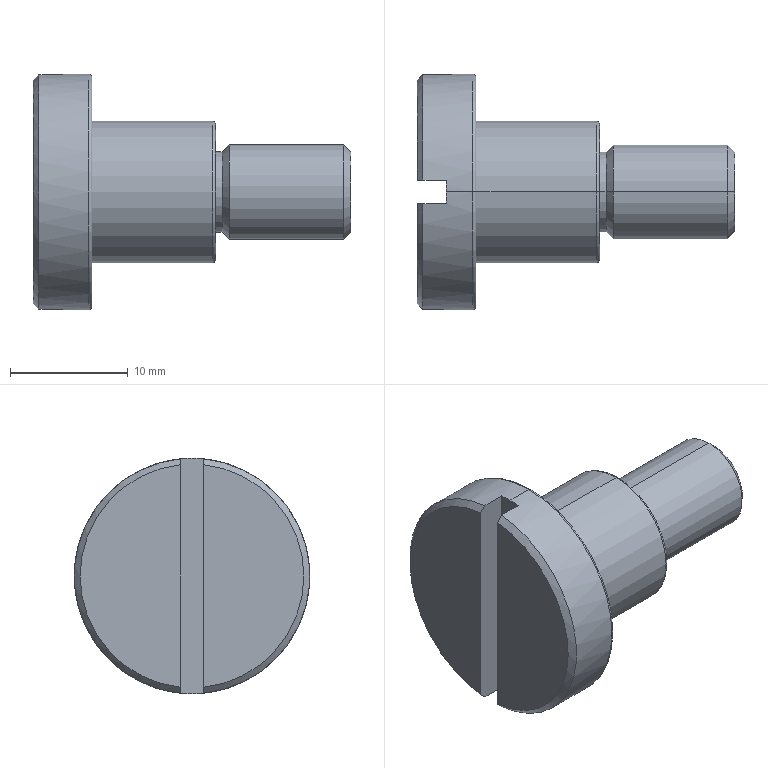Part | SolidWorks | features Chamfer 1, Fillet 1, ICE 1, Revolution 1 | 1 solid | 26 faces | box 27 x 20 x 20 mm | volume 3212 mm3 | cylinder 8 | plane 8 | cone 6 | torus 4 | commonest cylinder face diameters 6.8 x2 8 x2 12 x2 20 x2
STEP:
#1=CARTESIAN_POINT('',(5.,0.,-9.75));
#2=VERTEX_POINT('',#1);
#3=CARTESIAN_POINT('',(5.,0.,9.75));
#4=VERTEX_POINT('',#3);
#5=CARTESIAN_POINT('',(5.,0.,0.));
#6=DIRECTION('',(1.,0.,0.));
#7=DIRECTION('',(0.,0.,1.));
#8=AXIS2_PLACEMENT_3D('',#5,#6,#7);
#9=CIRCLE('',#8,9.75);
#10=EDGE_CURVE('',#2,#4,#9,.T.);
#11=ORIENTED_EDGE('',*,*,#10,.F.);
#12=CARTESIAN_POINT('',(4.75,0.,-10.));
#13=VERTEX_POINT('',#12);
#14=CARTESIAN_POINT('',(4.75,0.,-9.75));
#15=DIRECTION('',(0.,1.,0.));
#16=DIRECTION('',(0.,0.,1.));
#17=AXIS2_PLACEMENT_3D('',#14,#15,#16);
#18=CIRCLE('',#17,0.25);
#19=EDGE_CURVE('',#2,#13,#18,.T.);
#20=ORIENTED_EDGE('',*,*,#19,.T.);
#21=CARTESIAN_POINT('',(4.75,0.,10.));
#22=VERTEX_POINT('',#21);
#23=CARTESIAN_POINT('',(4.75,0.,0.));
#24=DIRECTION('',(-1.,0.,0.));
#25=DIRECTION('',(0.,0.,1.));
#26=AXIS2_PLACEMENT_3D('',#23,#24,#25);
#27=CIRCLE('',#26,10.);
#28=EDGE_CURVE('',#22,#13,#27,.T.);
#29=ORIENTED_EDGE('',*,*,#28,.F.);
#30=CARTESIAN_POINT('',(4.75,0.,9.75));
#31=DIRECTION('',(0.,-1.,0.));
#32=DIRECTION('',(0.,0.,-1.));
#33=AXIS2_PLACEMENT_3D('',#30,#31,#32);
#34=CIRCLE('',#33,0.25);
#35=EDGE_CURVE('',#4,#22,#34,.T.);
#36=ORIENTED_EDGE('',*,*,#35,.F.);
#37=EDGE_LOOP('',(#11,#20,#29,#36));
#38=FACE_OUTER_BOUND('',#37,.T.);
#39=CARTESIAN_POINT('',(4.75,0.,0.));
#40=DIRECTION('',(-1.,0.,0.));
#41=DIRECTION('',(0.,0.,1.));
#42=AXIS2_PLACEMENT_3D('',#39,#40,#41);
#43=TOROIDAL_SURFACE('',#42,9.75,0.25);
#44=ADVANCED_FACE('',(#38),#43,.T.);
#45=CARTESIAN_POINT('',(15.5,0.,-5.75));
#46=VERTEX_POINT('',#45);
#47=CARTESIAN_POINT('',(15.5,0.,5.75));
#48=VERTEX_POINT('',#47);
#49=CARTESIAN_POINT('',(15.5,0.,0.));
#50=DIRECTION('',(1.,0.,0.));
#51=DIRECTION('',(0.,0.,1.));
#52=AXIS2_PLACEMENT_3D('',#49,#50,#51);
#53=CIRCLE('',#52,5.75);
#54=EDGE_CURVE('',#46,#48,#53,.T.);
#55=ORIENTED_EDGE('',*,*,#54,.F.);
#56=CARTESIAN_POINT('',(15.25,0.,-6.));
#57=VERTEX_POINT('',#56);
#58=CARTESIAN_POINT('',(15.25,0.,-5.75));
#59=DIRECTION('',(0.,1.,0.));
#60=DIRECTION('',(0.,0.,1.));
#61=AXIS2_PLACEMENT_3D('',#58,#59,#60);
#62=CIRCLE('',#61,0.25);
#63=EDGE_CURVE('',#46,#57,#62,.T.);
#64=ORIENTED_EDGE('',*,*,#63,.T.);
#65=CARTESIAN_POINT('',(15.25,0.,6.));
#66=VERTEX_POINT('',#65);
#67=CARTESIAN_POINT('',(15.25,0.,0.));
#68=DIRECTION('',(-1.,0.,0.));
#69=DIRECTION('',(0.,0.,1.));
#70=AXIS2_PLACEMENT_3D('',#67,#68,#69);
#71=CIRCLE('',#70,6.);
#72=EDGE_CURVE('',#66,#57,#71,.T.);
#73=ORIENTED_EDGE('',*,*,#72,.F.);
#74=CARTESIAN_POINT('',(15.25,0.,5.75));
#75=DIRECTION('',(0.,-1.,0.));
#76=DIRECTION('',(0.,0.,-1.));
#77=AXIS2_PLACEMENT_3D('',#74,#75,#76);
#78=CIRCLE('',#77,0.25);
#79=EDGE_CURVE('',#48,#66,#78,.T.);
#80=ORIENTED_EDGE('',*,*,#79,.F.);
#81=EDGE_LOOP('',(#55,#64,#73,#80));
#82=FACE_OUTER_BOUND('',#81,.T.);
#83=CARTESIAN_POINT('',(15.25,0.,0.));
#84=DIRECTION('',(-1.,0.,0.));
#85=DIRECTION('',(0.,0.,1.));
#86=AXIS2_PLACEMENT_3D('',#83,#84,#85);
#87=TOROIDAL_SURFACE('',#86,5.75,0.25);
#88=ADVANCED_FACE('',(#82),#87,.T.);
#89=CARTESIAN_POINT('',(27.,0.,3.4));
#90=VERTEX_POINT('',#89);
#91=CARTESIAN_POINT('',(27.,0.,-3.4));
#92=VERTEX_POINT('',#91);
#93=CARTESIAN_POINT('',(27.,0.,0.));
#94=DIRECTION('',(-1.,0.,0.));
#95=DIRECTION('',(0.,0.,1.));
#96=AXIS2_PLACEMENT_3D('',#93,#94,#95);
#97=CIRCLE('',#96,3.4);
#98=EDGE_CURVE('',#90,#92,#97,.T.);
#99=ORIENTED_EDGE('',*,*,#98,.T.);
#100=CARTESIAN_POINT('',(26.4,0.,-4.));
#101=VERTEX_POINT('',#100);
#102=CARTESIAN_POINT('',(27.,0.,-3.4));
#103=DIRECTION('',(-0.7071,0.,-0.7071));
#104=VECTOR('',#103,1000.);
#105=LINE('',#102,#104);
#106=EDGE_CURVE('',#92,#101,#105,.T.);
#107=ORIENTED_EDGE('',*,*,#106,.T.);
#108=CARTESIAN_POINT('',(26.4,0.,4.));
#109=VERTEX_POINT('',#108);
#110=CARTESIAN_POINT('',(26.4,0.,0.));
#111=DIRECTION('',(-1.,0.,0.));
#112=DIRECTION('',(0.,0.,1.));
#113=AXIS2_PLACEMENT_3D('',#110,#111,#112);
#114=CIRCLE('',#113,4.);
#115=EDGE_CURVE('',#109,#101,#114,.T.);
#116=ORIENTED_EDGE('',*,*,#115,.F.);
#117=CARTESIAN_POINT('',(27.,0.,3.4));
#118=DIRECTION('',(-0.7071,0.,0.7071));
#119=VECTOR('',#118,1000.);
#120=LINE('',#117,#119);
#121=EDGE_CURVE('',#90,#109,#120,.T.);
#122=ORIENTED_EDGE('',*,*,#121,.F.);
#123=EDGE_LOOP('',(#99,#107,#116,#122));
#124=FACE_OUTER_BOUND('',#123,.T.);
#125=CARTESIAN_POINT('',(27.,0.,0.));
#126=DIRECTION('',(-1.,0.,0.));
#127=DIRECTION('',(0.,0.,1.));
#128=AXIS2_PLACEMENT_3D('',#125,#126,#127);
#129=CONICAL_SURFACE('',#128,3.4,0.7854);
#130=ADVANCED_FACE('',(#124),#129,.T.);
#131=ORIENTED_EDGE('',*,*,#115,.T.);
#132=CARTESIAN_POINT('',(16.65,0.,-4.));
#133=VERTEX_POINT('',#132);
#134=CARTESIAN_POINT('',(0.,0.,-4.));
#135=DIRECTION('',(-1.,0.,0.));
#136=VECTOR('',#135,1000.);
#137=LINE('',#134,#136);
#138=EDGE_CURVE('',#101,#133,#137,.T.);
#139=ORIENTED_EDGE('',*,*,#138,.T.);
#140=CARTESIAN_POINT('',(16.65,0.,4.));
#141=VERTEX_POINT('',#140);
#142=CARTESIAN_POINT('',(16.65,0.,0.));
#143=DIRECTION('',(-1.,0.,0.));
#144=DIRECTION('',(0.,0.,1.));
#145=AXIS2_PLACEMENT_3D('',#142,#143,#144);
#146=CIRCLE('',#145,4.);
#147=EDGE_CURVE('',#141,#133,#146,.T.);
#148=ORIENTED_EDGE('',*,*,#147,.F.);
#149=CARTESIAN_POINT('',(0.,0.,4.));
#150=DIRECTION('',(-1.,0.,0.));
#151=VECTOR('',#150,1000.);
#152=LINE('',#149,#151);
#153=EDGE_CURVE('',#109,#141,#152,.T.);
#154=ORIENTED_EDGE('',*,*,#153,.F.);
#155=EDGE_LOOP('',(#131,#139,#148,#154));
#156=FACE_OUTER_BOUND('',#155,.T.);
#157=CARTESIAN_POINT('',(0.,0.,0.));
#158=DIRECTION('',(-1.,0.,0.));
#159=DIRECTION('',(0.,0.,1.));
#160=AXIS2_PLACEMENT_3D('',#157,#158,#159);
#161=CYLINDRICAL_SURFACE('',#160,4.);
#162=ADVANCED_FACE('',(#156),#161,.T.);
#163=CARTESIAN_POINT('',(16.05,0.,3.4));
#164=VERTEX_POINT('',#163);
#165=CARTESIAN_POINT('',(16.05,0.,-3.4));
#166=VERTEX_POINT('',#165);
#167=CARTESIAN_POINT('',(16.05,0.,0.));
#168=DIRECTION('',(-1.,0.,0.));
#169=DIRECTION('',(0.,0.,1.));
#170=AXIS2_PLACEMENT_3D('',#167,#168,#169);
#171=CIRCLE('',#170,3.4);
#172=EDGE_CURVE('',#164,#166,#171,.T.);
#173=ORIENTED_EDGE('',*,*,#172,.F.);
#174=CARTESIAN_POINT('',(16.65,0.,4.));
#175=DIRECTION('',(0.7071,0.,0.7071));
#176=VECTOR('',#175,1000.);
#177=LINE('',#174,#176);
#178=EDGE_CURVE('',#164,#141,#177,.T.);
#179=ORIENTED_EDGE('',*,*,#178,.T.);
#180=ORIENTED_EDGE('',*,*,#147,.T.);
#181=CARTESIAN_POINT('',(16.65,0.,-4.));
#182=DIRECTION('',(0.7071,0.,-0.7071));
#183=VECTOR('',#182,1000.);
#184=LINE('',#181,#183);
#185=EDGE_CURVE('',#166,#133,#184,.T.);
#186=ORIENTED_EDGE('',*,*,#185,.F.);
#187=EDGE_LOOP('',(#173,#179,#180,#186));
#188=FACE_OUTER_BOUND('',#187,.T.);
#189=CARTESIAN_POINT('',(16.65,0.,0.));
#190=DIRECTION('',(1.,0.,0.));
#191=DIRECTION('',(0.,0.,-1.));
#192=AXIS2_PLACEMENT_3D('',#189,#190,#191);
#193=CONICAL_SURFACE('',#192,4.,0.7854);
#194=ADVANCED_FACE('',(#188),#193,.T.);
#195=ORIENTED_EDGE('',*,*,#172,.T.);
#196=CARTESIAN_POINT('',(15.5,0.,-3.4));
#197=VERTEX_POINT('',#196);
#198=CARTESIAN_POINT('',(0.,0.,-3.4));
#199=DIRECTION('',(-1.,0.,0.));
#200=VECTOR('',#199,1000.);
#201=LINE('',#198,#200);
#202=EDGE_CURVE('',#166,#197,#201,.T.);
#203=ORIENTED_EDGE('',*,*,#202,.T.);
#204=CARTESIAN_POINT('',(15.5,0.,3.4));
#205=VERTEX_POINT('',#204);
#206=CARTESIAN_POINT('',(15.5,0.,0.));
#207=DIRECTION('',(-1.,0.,0.));
#208=DIRECTION('',(0.,0.,1.));
#209=AXIS2_PLACEMENT_3D('',#206,#207,#208);
#210=CIRCLE('',#209,3.4);
#211=EDGE_CURVE('',#205,#197,#210,.T.);
#212=ORIENTED_EDGE('',*,*,#211,.F.);
#213=CARTESIAN_POINT('',(0.,0.,3.4));
#214=DIRECTION('',(-1.,0.,0.));
#215=VECTOR('',#214,1000.);
#216=LINE('',#213,#215);
#217=EDGE_CURVE('',#164,#205,#216,.T.);
#218=ORIENTED_EDGE('',*,*,#217,.F.);
#219=EDGE_LOOP('',(#195,#203,#212,#218));
#220=FACE_OUTER_BOUND('',#219,.T.);
#221=CARTESIAN_POINT('',(0.,0.,0.));
#222=DIRECTION('',(-1.,0.,0.));
#223=DIRECTION('',(0.,0.,1.));
#224=AXIS2_PLACEMENT_3D('',#221,#222,#223);
#225=CYLINDRICAL_SURFACE('',#224,3.4);
#226=ADVANCED_FACE('',(#220),#225,.T.);
#227=ORIENTED_EDGE('',*,*,#72,.T.);
#228=CARTESIAN_POINT('',(5.,0.,-6.));
#229=VERTEX_POINT('',#228);
#230=CARTESIAN_POINT('',(0.,0.,-6.));
#231=DIRECTION('',(-1.,0.,0.));
#232=VECTOR('',#231,1000.);
#233=LINE('',#230,#232);
#234=EDGE_CURVE('',#57,#229,#233,.T.);
#235=ORIENTED_EDGE('',*,*,#234,.T.);
#236=CARTESIAN_POINT('',(5.,0.,6.));
#237=VERTEX_POINT('',#236);
#238=CARTESIAN_POINT('',(5.,0.,0.));
#239=DIRECTION('',(-1.,0.,0.));
#240=DIRECTION('',(0.,0.,1.));
#241=AXIS2_PLACEMENT_3D('',#238,#239,#240);
#242=CIRCLE('',#241,6.);
#243=EDGE_CURVE('',#237,#229,#242,.T.);
#244=ORIENTED_EDGE('',*,*,#243,.F.);
#245=CARTESIAN_POINT('',(0.,0.,6.));
#246=DIRECTION('',(-1.,0.,0.));
#247=VECTOR('',#246,1000.);
#248=LINE('',#245,#247);
#249=EDGE_CURVE('',#66,#237,#248,.T.);
#250=ORIENTED_EDGE('',*,*,#249,.F.);
#251=EDGE_LOOP('',(#227,#235,#244,#250));
#252=FACE_OUTER_BOUND('',#251,.T.);
#253=CARTESIAN_POINT('',(0.,0.,0.));
#254=DIRECTION('',(-1.,0.,0.));
#255=DIRECTION('',(0.,0.,1.));
#256=AXIS2_PLACEMENT_3D('',#253,#254,#255);
#257=CYLINDRICAL_SURFACE('',#256,6.);
#258=ADVANCED_FACE('',(#252),#257,.T.);
#259=ORIENTED_EDGE('',*,*,#28,.T.);
#260=CARTESIAN_POINT('',(2.5,0.,-10.));
#261=VERTEX_POINT('',#260);
#262=CARTESIAN_POINT('',(0.,0.,-10.));
#263=DIRECTION('',(-1.,0.,0.));
#264=VECTOR('',#263,1000.);
#265=LINE('',#262,#264);
#266=EDGE_CURVE('',#13,#261,#265,.T.);
#267=ORIENTED_EDGE('',*,*,#266,.T.);
#268=CARTESIAN_POINT('',(2.5,1.,-9.95));
#269=VERTEX_POINT('',#268);
#270=CARTESIAN_POINT('',(2.5,0.,0.));
#271=DIRECTION('',(1.,0.,0.));
#272=DIRECTION('',(0.,0.,-1.));
#273=AXIS2_PLACEMENT_3D('',#270,#271,#272);
#274=CIRCLE('',#273,10.);
#275=EDGE_CURVE('',#261,#269,#274,.T.);
#276=ORIENTED_EDGE('',*,*,#275,.T.);
#277=CARTESIAN_POINT('',(0.5,1.,-9.95));
#278=VERTEX_POINT('',#277);
#279=CARTESIAN_POINT('',(0.,1.,-9.95));
#280=DIRECTION('',(-1.,0.,0.));
#281=VECTOR('',#280,1000.);
#282=LINE('',#279,#281);
#283=EDGE_CURVE('',#269,#278,#282,.T.);
#284=ORIENTED_EDGE('',*,*,#283,.T.);
#285=CARTESIAN_POINT('',(0.5,1.,9.95));
#286=VERTEX_POINT('',#285);
#287=CARTESIAN_POINT('',(0.5,0.,0.));
#288=DIRECTION('',(1.,0.,0.));
#289=DIRECTION('',(0.,0.,-1.));
#290=AXIS2_PLACEMENT_3D('',#287,#288,#289);
#291=CIRCLE('',#290,10.);
#292=EDGE_CURVE('',#278,#286,#291,.T.);
#293=ORIENTED_EDGE('',*,*,#292,.T.);
#294=CARTESIAN_POINT('',(2.5,1.,9.95));
#295=VERTEX_POINT('',#294);
#296=CARTESIAN_POINT('',(0.,1.,9.95));
#297=DIRECTION('',(1.,0.,0.));
#298=VECTOR('',#297,1000.);
#299=LINE('',#296,#298);
#300=EDGE_CURVE('',#286,#295,#299,.T.);
#301=ORIENTED_EDGE('',*,*,#300,.T.);
#302=CARTESIAN_POINT('',(2.5,0.,10.));
#303=VERTEX_POINT('',#302);
#304=CARTESIAN_POINT('',(2.5,0.,0.));
#305=DIRECTION('',(1.,0.,0.));
#306=DIRECTION('',(0.,0.,-1.));
#307=AXIS2_PLACEMENT_3D('',#304,#305,#306);
#308=CIRCLE('',#307,10.);
#309=EDGE_CURVE('',#295,#303,#308,.T.);
#310=ORIENTED_EDGE('',*,*,#309,.T.);
#311=CARTESIAN_POINT('',(0.,0.,10.));
#312=DIRECTION('',(-1.,0.,0.));
#313=VECTOR('',#312,1000.);
#314=LINE('',#311,#313);
#315=EDGE_CURVE('',#22,#303,#314,.T.);
#316=ORIENTED_EDGE('',*,*,#315,.F.);
#317=EDGE_LOOP('',(#259,#267,#276,#284,#293,#301,#310,#316));
#318=FACE_OUTER_BOUND('',#317,.T.);
#319=CARTESIAN_POINT('',(0.,0.,0.));
#320=DIRECTION('',(-1.,0.,0.));
#321=DIRECTION('',(0.,0.,1.));
#322=AXIS2_PLACEMENT_3D('',#319,#320,#321);
#323=CYLINDRICAL_SURFACE('',#322,10.);
#324=ADVANCED_FACE('',(#318),#323,.T.);
#325=CARTESIAN_POINT('',(0.,1.,9.447));
#326=VERTEX_POINT('',#325);
#327=CARTESIAN_POINT('',(0.,1.,-9.447));
#328=VERTEX_POINT('',#327);
#329=CARTESIAN_POINT('',(0.,0.,0.));
#330=DIRECTION('',(-1.,0.,0.));
#331=DIRECTION('',(0.,0.,-1.));
#332=AXIS2_PLACEMENT_3D('',#329,#330,#331);
#333=CIRCLE('',#332,9.5);
#334=EDGE_CURVE('',#326,#328,#333,.T.);
#335=ORIENTED_EDGE('',*,*,#334,.T.);
#336=CARTESIAN_POINT('',(0.,1.,-10.));
#337=DIRECTION('',(0.,0.,1.));
#338=VECTOR('',#337,1000.);
#339=LINE('',#336,#338);
#340=EDGE_CURVE('',#328,#326,#339,.T.);
#341=ORIENTED_EDGE('',*,*,#340,.T.);
#342=EDGE_LOOP('',(#335,#341));
#343=FACE_OUTER_BOUND('',#342,.T.);
#344=CARTESIAN_POINT('',(0.,0.,0.));
#345=DIRECTION('',(1.,0.,0.));
#346=DIRECTION('',(0.,0.,-1.));
#347=AXIS2_PLACEMENT_3D('',#344,#345,#346);
#348=PLANE('',#347);
#349=ADVANCED_FACE('',(#343),#348,.F.);
#350=CARTESIAN_POINT('',(0.5,1.,9.95));
#351=CARTESIAN_POINT('',(0.3333,1.,9.782));
#352=CARTESIAN_POINT('',(0.1666,1.,9.615));
#353=CARTESIAN_POINT('',(0.,1.,9.447));
#354=B_SPLINE_CURVE_WITH_KNOTS('',3,(#350,#351,#352,#353),.UNSPECIFIED.,.F.,.F.,(4,4),(0.017,0.0177),.UNSPECIFIED.);
#355=EDGE_CURVE('',#286,#326,#354,.T.);
#356=ORIENTED_EDGE('',*,*,#355,.F.);
#357=ORIENTED_EDGE('',*,*,#292,.F.);
#358=CARTESIAN_POINT('',(0.,1.,-9.447));
#359=CARTESIAN_POINT('',(0.1666,1.,-9.615));
#360=CARTESIAN_POINT('',(0.3333,1.,-9.782));
#361=CARTESIAN_POINT('',(0.5,1.,-9.95));
#362=B_SPLINE_CURVE_WITH_KNOTS('',3,(#358,#359,#360,#361),.UNSPECIFIED.,.F.,.F.,(4,4),(0.04341,0.04413),.UNSPECIFIED.);
#363=EDGE_CURVE('',#328,#278,#362,.T.);
#364=ORIENTED_EDGE('',*,*,#363,.F.);
#365=ORIENTED_EDGE('',*,*,#334,.F.);
#366=EDGE_LOOP('',(#356,#357,#364,#365));
#367=FACE_OUTER_BOUND('',#366,.T.);
#368=CARTESIAN_POINT('',(0.,0.,0.));
#369=DIRECTION('',(1.,0.,0.));
#370=DIRECTION('',(0.,0.,-1.));
#371=AXIS2_PLACEMENT_3D('',#368,#369,#370);
#372=CONICAL_SURFACE('',#371,9.5,0.7854);
#373=ADVANCED_FACE('',(#367),#372,.T.);
#374=CARTESIAN_POINT('',(0.,-1.,-9.447));
#375=VERTEX_POINT('',#374);
#376=CARTESIAN_POINT('',(0.,-1.,9.447));
#377=VERTEX_POINT('',#376);
#378=CARTESIAN_POINT('',(0.,0.,0.));
#379=DIRECTION('',(-1.,0.,0.));
#380=DIRECTION('',(0.,0.,-1.));
#381=AXIS2_PLACEMENT_3D('',#378,#379,#380);
#382=CIRCLE('',#381,9.5);
#383=EDGE_CURVE('',#375,#377,#382,.T.);
#384=ORIENTED_EDGE('',*,*,#383,.T.);
#385=CARTESIAN_POINT('',(0.,-1.,-10.));
#386=DIRECTION('',(0.,0.,1.));
#387=VECTOR('',#386,1000.);
#388=LINE('',#385,#387);
#389=EDGE_CURVE('',#375,#377,#388,.T.);
#390=ORIENTED_EDGE('',*,*,#389,.F.);
#391=EDGE_LOOP('',(#384,#390));
#392=FACE_OUTER_BOUND('',#391,.T.);
#393=CARTESIAN_POINT('',(0.,0.,0.));
#394=DIRECTION('',(1.,0.,0.));
#395=DIRECTION('',(0.,0.,-1.));
#396=AXIS2_PLACEMENT_3D('',#393,#394,#395);
#397=PLANE('',#396);
#398=ADVANCED_FACE('',(#392),#397,.F.);
#399=ORIENTED_EDGE('',*,*,#266,.F.);
#400=CARTESIAN_POINT('',(4.75,0.,0.));
#401=DIRECTION('',(-1.,0.,0.));
#402=DIRECTION('',(0.,0.,1.));
#403=AXIS2_PLACEMENT_3D('',#400,#401,#402);
#404=CIRCLE('',#403,10.);
#405=EDGE_CURVE('',#13,#22,#404,.T.);
#406=ORIENTED_EDGE('',*,*,#405,.T.);
#407=ORIENTED_EDGE('',*,*,#315,.T.);
#408=CARTESIAN_POINT('',(2.5,-1.,9.95));
#409=VERTEX_POINT('',#408);
#410=CARTESIAN_POINT('',(2.5,0.,0.));
#411=DIRECTION('',(1.,0.,0.));
#412=DIRECTION('',(0.,0.,-1.));
#413=AXIS2_PLACEMENT_3D('',#410,#411,#412);
#414=CIRCLE('',#413,10.);
#415=EDGE_CURVE('',#303,#409,#414,.T.);
#416=ORIENTED_EDGE('',*,*,#415,.T.);
#417=CARTESIAN_POINT('',(0.5,-1.,9.95));
#418=VERTEX_POINT('',#417);
#419=CARTESIAN_POINT('',(0.,-1.,9.95));
#420=DIRECTION('',(-1.,0.,0.));
#421=VECTOR('',#420,1000.);
#422=LINE('',#419,#421);
#423=EDGE_CURVE('',#409,#418,#422,.T.);
#424=ORIENTED_EDGE('',*,*,#423,.T.);
#425=CARTESIAN_POINT('',(0.5,-1.,-9.95));
#426=VERTEX_POINT('',#425);
#427=CARTESIAN_POINT('',(0.5,0.,0.));
#428=DIRECTION('',(1.,0.,0.));
#429=DIRECTION('',(0.,0.,-1.));
#430=AXIS2_PLACEMENT_3D('',#427,#428,#429);
#431=CIRCLE('',#430,10.);
#432=EDGE_CURVE('',#418,#426,#431,.T.);
#433=ORIENTED_EDGE('',*,*,#432,.T.);
#434=CARTESIAN_POINT('',(2.5,-1.,-9.95));
#435=VERTEX_POINT('',#434);
#436=CARTESIAN_POINT('',(0.,-1.,-9.95));
#437=DIRECTION('',(1.,0.,0.));
#438=VECTOR('',#437,1000.);
#439=LINE('',#436,#438);
#440=EDGE_CURVE('',#426,#435,#439,.T.);
#441=ORIENTED_EDGE('',*,*,#440,.T.);
#442=CARTESIAN_POINT('',(2.5,0.,0.));
#443=DIRECTION('',(1.,0.,0.));
#444=DIRECTION('',(0.,0.,-1.));
#445=AXIS2_PLACEMENT_3D('',#442,#443,#444);
#446=CIRCLE('',#445,10.);
#447=EDGE_CURVE('',#435,#261,#446,.T.);
#448=ORIENTED_EDGE('',*,*,#447,.T.);
#449=EDGE_LOOP('',(#399,#406,#407,#416,#424,#433,#441,#448));
#450=FACE_OUTER_BOUND('',#449,.T.);
#451=CARTESIAN_POINT('',(0.,0.,0.));
#452=DIRECTION('',(-1.,0.,0.));
#453=DIRECTION('',(0.,0.,1.));
#454=AXIS2_PLACEMENT_3D('',#451,#452,#453);
#455=CYLINDRICAL_SURFACE('',#454,10.);
#456=ADVANCED_FACE('',(#450),#455,.T.);
#457=CARTESIAN_POINT('',(5.,0.,0.));
#458=DIRECTION('',(1.,0.,0.));
#459=DIRECTION('',(0.,0.,1.));
#460=AXIS2_PLACEMENT_3D('',#457,#458,#459);
#461=CIRCLE('',#460,9.75);
#462=EDGE_CURVE('',#4,#2,#461,.T.);
#463=ORIENTED_EDGE('',*,*,#462,.T.);
#464=ORIENTED_EDGE('',*,*,#10,.T.);
#465=EDGE_LOOP('',(#463,#464));
#466=FACE_OUTER_BOUND('',#465,.T.);
#467=ORIENTED_EDGE('',*,*,#243,.T.);
#468=CARTESIAN_POINT('',(5.,0.,0.));
#469=DIRECTION('',(-1.,0.,0.));
#470=DIRECTION('',(0.,0.,1.));
#471=AXIS2_PLACEMENT_3D('',#468,#469,#470);
#472=CIRCLE('',#471,6.);
#473=EDGE_CURVE('',#229,#237,#472,.T.);
#474=ORIENTED_EDGE('',*,*,#473,.T.);
#475=EDGE_LOOP('',(#467,#474));
#476=FACE_BOUND('',#475,.T.);
#477=CARTESIAN_POINT('',(5.,-10.,0.));
#478=DIRECTION('',(-1.,0.,0.));
#479=DIRECTION('',(0.,0.,1.));
#480=AXIS2_PLACEMENT_3D('',#477,#478,#479);
#481=PLANE('',#480);
#482=ADVANCED_FACE('',(#466,#476),#481,.F.);
#483=ORIENTED_EDGE('',*,*,#234,.F.);
#484=CARTESIAN_POINT('',(15.25,0.,0.));
#485=DIRECTION('',(-1.,0.,0.));
#486=DIRECTION('',(0.,0.,1.));
#487=AXIS2_PLACEMENT_3D('',#484,#485,#486);
#488=CIRCLE('',#487,6.);
#489=EDGE_CURVE('',#57,#66,#488,.T.);
#490=ORIENTED_EDGE('',*,*,#489,.T.);
#491=ORIENTED_EDGE('',*,*,#249,.T.);
#492=ORIENTED_EDGE('',*,*,#473,.F.);
#493=EDGE_LOOP('',(#483,#490,#491,#492));
#494=FACE_OUTER_BOUND('',#493,.T.);
#495=CARTESIAN_POINT('',(0.,0.,0.));
#496=DIRECTION('',(-1.,0.,0.));
#497=DIRECTION('',(0.,0.,1.));
#498=AXIS2_PLACEMENT_3D('',#495,#496,#497);
#499=CYLINDRICAL_SURFACE('',#498,6.);
#500=ADVANCED_FACE('',(#494),#499,.T.);
#501=CARTESIAN_POINT('',(15.5,0.,0.));
#502=DIRECTION('',(1.,0.,0.));
#503=DIRECTION('',(0.,0.,1.));
#504=AXIS2_PLACEMENT_3D('',#501,#502,#503);
#505=CIRCLE('',#504,5.75);
#506=EDGE_CURVE('',#48,#46,#505,.T.);
#507=ORIENTED_EDGE('',*,*,#506,.T.);
#508=ORIENTED_EDGE('',*,*,#54,.T.);
#509=EDGE_LOOP('',(#507,#508));
#510=FACE_OUTER_BOUND('',#509,.T.);
#511=ORIENTED_EDGE('',*,*,#211,.T.);
#512=CARTESIAN_POINT('',(15.5,0.,0.));
#513=DIRECTION('',(-1.,0.,0.));
#514=DIRECTION('',(0.,0.,1.));
#515=AXIS2_PLACEMENT_3D('',#512,#513,#514);
#516=CIRCLE('',#515,3.4);
#517=EDGE_CURVE('',#197,#205,#516,.T.);
#518=ORIENTED_EDGE('',*,*,#517,.T.);
#519=EDGE_LOOP('',(#511,#518));
#520=FACE_BOUND('',#519,.T.);
#521=CARTESIAN_POINT('',(15.5,-4.,0.));
#522=DIRECTION('',(-1.,0.,0.));
#523=DIRECTION('',(0.,0.,1.));
#524=AXIS2_PLACEMENT_3D('',#521,#522,#523);
#525=PLANE('',#524);
#526=ADVANCED_FACE('',(#510,#520),#525,.F.);
#527=ORIENTED_EDGE('',*,*,#202,.F.);
#528=CARTESIAN_POINT('',(16.05,0.,0.));
#529=DIRECTION('',(-1.,0.,0.));
#530=DIRECTION('',(0.,0.,1.));
#531=AXIS2_PLACEMENT_3D('',#528,#529,#530);
#532=CIRCLE('',#531,3.4);
#533=EDGE_CURVE('',#166,#164,#532,.T.);
#534=ORIENTED_EDGE('',*,*,#533,.T.);
#535=ORIENTED_EDGE('',*,*,#217,.T.);
#536=ORIENTED_EDGE('',*,*,#517,.F.);
#537=EDGE_LOOP('',(#527,#534,#535,#536));
#538=FACE_OUTER_BOUND('',#537,.T.);
#539=CARTESIAN_POINT('',(0.,0.,0.));
#540=DIRECTION('',(-1.,0.,0.));
#541=DIRECTION('',(0.,0.,1.));
#542=AXIS2_PLACEMENT_3D('',#539,#540,#541);
#543=CYLINDRICAL_SURFACE('',#542,3.4);
#544=ADVANCED_FACE('',(#538),#543,.T.);
#545=ORIENTED_EDGE('',*,*,#178,.F.);
#546=ORIENTED_EDGE('',*,*,#533,.F.);
#547=ORIENTED_EDGE('',*,*,#185,.T.);
#548=CARTESIAN_POINT('',(16.65,0.,0.));
#549=DIRECTION('',(-1.,0.,0.));
#550=DIRECTION('',(0.,0.,1.));
#551=AXIS2_PLACEMENT_3D('',#548,#549,#550);
#552=CIRCLE('',#551,4.);
#553=EDGE_CURVE('',#133,#141,#552,.T.);
#554=ORIENTED_EDGE('',*,*,#553,.T.);
#555=EDGE_LOOP('',(#545,#546,#547,#554));
#556=FACE_OUTER_BOUND('',#555,.T.);
#557=CARTESIAN_POINT('',(16.65,0.,0.));
#558=DIRECTION('',(1.,0.,0.));
#559=DIRECTION('',(0.,0.,-1.));
#560=AXIS2_PLACEMENT_3D('',#557,#558,#559);
#561=CONICAL_SURFACE('',#560,4.,0.7854);
#562=ADVANCED_FACE('',(#556),#561,.T.);
#563=ORIENTED_EDGE('',*,*,#138,.F.);
#564=CARTESIAN_POINT('',(26.4,0.,0.));
#565=DIRECTION('',(-1.,0.,0.));
#566=DIRECTION('',(0.,0.,1.));
#567=AXIS2_PLACEMENT_3D('',#564,#565,#566);
#568=CIRCLE('',#567,4.);
#569=EDGE_CURVE('',#101,#109,#568,.T.);
#570=ORIENTED_EDGE('',*,*,#569,.T.);
#571=ORIENTED_EDGE('',*,*,#153,.T.);
#572=ORIENTED_EDGE('',*,*,#553,.F.);
#573=EDGE_LOOP('',(#563,#570,#571,#572));
#574=FACE_OUTER_BOUND('',#573,.T.);
#575=CARTESIAN_POINT('',(0.,0.,0.));
#576=DIRECTION('',(-1.,0.,0.));
#577=DIRECTION('',(0.,0.,1.));
#578=AXIS2_PLACEMENT_3D('',#575,#576,#577);
#579=CYLINDRICAL_SURFACE('',#578,4.);
#580=ADVANCED_FACE('',(#574),#579,.T.);
#581=ORIENTED_EDGE('',*,*,#106,.F.);
#582=CARTESIAN_POINT('',(27.,0.,0.));
#583=DIRECTION('',(-1.,0.,0.));
#584=DIRECTION('',(0.,0.,1.));
#585=AXIS2_PLACEMENT_3D('',#582,#583,#584);
#586=CIRCLE('',#585,3.4);
#587=EDGE_CURVE('',#92,#90,#586,.T.);
#588=ORIENTED_EDGE('',*,*,#587,.T.);
#589=ORIENTED_EDGE('',*,*,#121,.T.);
#590=ORIENTED_EDGE('',*,*,#569,.F.);
#591=EDGE_LOOP('',(#581,#588,#589,#590));
#592=FACE_OUTER_BOUND('',#591,.T.);
#593=CARTESIAN_POINT('',(27.,0.,0.));
#594=DIRECTION('',(-1.,0.,0.));
#595=DIRECTION('',(0.,0.,1.));
#596=AXIS2_PLACEMENT_3D('',#593,#594,#595);
#597=CONICAL_SURFACE('',#596,3.4,0.7854);
#598=ADVANCED_FACE('',(#592),#597,.T.);
#599=ORIENTED_EDGE('',*,*,#98,.F.);
#600=ORIENTED_EDGE('',*,*,#587,.F.);
#601=EDGE_LOOP('',(#599,#600));
#602=FACE_OUTER_BOUND('',#601,.T.);
#603=CARTESIAN_POINT('',(27.,-3.4,0.));
#604=DIRECTION('',(-1.,0.,0.));
#605=DIRECTION('',(0.,0.,1.));
#606=AXIS2_PLACEMENT_3D('',#603,#604,#605);
#607=PLANE('',#606);
#608=ADVANCED_FACE('',(#602),#607,.F.);
#609=CARTESIAN_POINT('',(0.5,-1.,-9.95));
#610=CARTESIAN_POINT('',(0.3333,-1.,-9.782));
#611=CARTESIAN_POINT('',(0.1666,-1.,-9.615));
#612=CARTESIAN_POINT('',(0.,-1.,-9.447));
#613=B_SPLINE_CURVE_WITH_KNOTS('',3,(#609,#610,#611,#612),.UNSPECIFIED.,.F.,.F.,(4,4),(0.017,0.0177),.UNSPECIFIED.);
#614=EDGE_CURVE('',#426,#375,#613,.T.);
#615=ORIENTED_EDGE('',*,*,#614,.F.);
#616=ORIENTED_EDGE('',*,*,#432,.F.);
#617=CARTESIAN_POINT('',(0.,-1.,9.447));
#618=CARTESIAN_POINT('',(0.1666,-1.,9.615));
#619=CARTESIAN_POINT('',(0.3333,-1.,9.782));
#620=CARTESIAN_POINT('',(0.5,-1.,9.95));
#621=B_SPLINE_CURVE_WITH_KNOTS('',3,(#617,#618,#619,#620),.UNSPECIFIED.,.F.,.F.,(4,4),(0.04341,0.04413),.UNSPECIFIED.);
#622=EDGE_CURVE('',#377,#418,#621,.T.);
#623=ORIENTED_EDGE('',*,*,#622,.F.);
#624=ORIENTED_EDGE('',*,*,#383,.F.);
#625=EDGE_LOOP('',(#615,#616,#623,#624));
#626=FACE_OUTER_BOUND('',#625,.T.);
#627=CARTESIAN_POINT('',(0.,0.,0.));
#628=DIRECTION('',(1.,0.,0.));
#629=DIRECTION('',(0.,0.,-1.));
#630=AXIS2_PLACEMENT_3D('',#627,#628,#629);
#631=CONICAL_SURFACE('',#630,9.5,0.7854);
#632=ADVANCED_FACE('',(#626),#631,.T.);
#633=CARTESIAN_POINT('',(2.5,1.,-10.));
#634=DIRECTION('',(0.,0.,1.));
#635=VECTOR('',#634,1000.);
#636=LINE('',#633,#635);
#637=EDGE_CURVE('',#269,#295,#636,.T.);
#638=ORIENTED_EDGE('',*,*,#637,.F.);
#639=ORIENTED_EDGE('',*,*,#275,.F.);
#640=ORIENTED_EDGE('',*,*,#447,.F.);
#641=CARTESIAN_POINT('',(2.5,-1.,-10.));
#642=DIRECTION('',(0.,0.,1.));
#643=VECTOR('',#642,1000.);
#644=LINE('',#641,#643);
#645=EDGE_CURVE('',#435,#409,#644,.T.);
#646=ORIENTED_EDGE('',*,*,#645,.T.);
#647=ORIENTED_EDGE('',*,*,#415,.F.);
#648=ORIENTED_EDGE('',*,*,#309,.F.);
#649=EDGE_LOOP('',(#638,#639,#640,#646,#647,#648));
#650=FACE_OUTER_BOUND('',#649,.T.);
#651=CARTESIAN_POINT('',(2.5,1.,-10.));
#652=DIRECTION('',(1.,0.,0.));
#653=DIRECTION('',(0.,0.,-1.));
#654=AXIS2_PLACEMENT_3D('',#651,#652,#653);
#655=PLANE('',#654);
#656=ADVANCED_FACE('',(#650),#655,.F.);
#657=ORIENTED_EDGE('',*,*,#355,.T.);
#658=ORIENTED_EDGE('',*,*,#340,.F.);
#659=ORIENTED_EDGE('',*,*,#363,.T.);
#660=ORIENTED_EDGE('',*,*,#283,.F.);
#661=ORIENTED_EDGE('',*,*,#637,.T.);
#662=ORIENTED_EDGE('',*,*,#300,.F.);
#663=EDGE_LOOP('',(#657,#658,#659,#660,#661,#662));
#664=FACE_OUTER_BOUND('',#663,.T.);
#665=CARTESIAN_POINT('',(0.,1.,-10.));
#666=DIRECTION('',(0.,1.,0.));
#667=DIRECTION('',(0.,0.,1.));
#668=AXIS2_PLACEMENT_3D('',#665,#666,#667);
#669=PLANE('',#668);
#670=ADVANCED_FACE('',(#664),#669,.F.);
#671=ORIENTED_EDGE('',*,*,#614,.T.);
#672=ORIENTED_EDGE('',*,*,#389,.T.);
#673=ORIENTED_EDGE('',*,*,#622,.T.);
#674=ORIENTED_EDGE('',*,*,#423,.F.);
#675=ORIENTED_EDGE('',*,*,#645,.F.);
#676=ORIENTED_EDGE('',*,*,#440,.F.);
#677=EDGE_LOOP('',(#671,#672,#673,#674,#675,#676));
#678=FACE_OUTER_BOUND('',#677,.T.);
#679=CARTESIAN_POINT('',(0.,-1.,-10.));
#680=DIRECTION('',(0.,-1.,0.));
#681=DIRECTION('',(1.,0.,0.));
#682=AXIS2_PLACEMENT_3D('',#679,#680,#681);
#683=PLANE('',#682);
#684=ADVANCED_FACE('',(#678),#683,.F.);
#685=ORIENTED_EDGE('',*,*,#63,.F.);
#686=ORIENTED_EDGE('',*,*,#506,.F.);
#687=ORIENTED_EDGE('',*,*,#79,.T.);
#688=ORIENTED_EDGE('',*,*,#489,.F.);
#689=EDGE_LOOP('',(#685,#686,#687,#688));
#690=FACE_OUTER_BOUND('',#689,.T.);
#691=CARTESIAN_POINT('',(15.25,0.,0.));
#692=DIRECTION('',(-1.,0.,0.));
#693=DIRECTION('',(0.,0.,1.));
#694=AXIS2_PLACEMENT_3D('',#691,#692,#693);
#695=TOROIDAL_SURFACE('',#694,5.75,0.25);
#696=ADVANCED_FACE('',(#690),#695,.T.);
#697=ORIENTED_EDGE('',*,*,#19,.F.);
#698=ORIENTED_EDGE('',*,*,#462,.F.);
#699=ORIENTED_EDGE('',*,*,#35,.T.);
#700=ORIENTED_EDGE('',*,*,#405,.F.);
#701=EDGE_LOOP('',(#697,#698,#699,#700));
#702=FACE_OUTER_BOUND('',#701,.T.);
#703=CARTESIAN_POINT('',(4.75,0.,0.));
#704=DIRECTION('',(-1.,0.,0.));
#705=DIRECTION('',(0.,0.,1.));
#706=AXIS2_PLACEMENT_3D('',#703,#704,#705);
#707=TOROIDAL_SURFACE('',#706,9.75,0.25);
#708=ADVANCED_FACE('',(#702),#707,.T.);
#709=CLOSED_SHELL('',(#44,#88,#130,#162,#194,#226,#258,#324,#349,#373,#398,#456,#482,#500,#526,#544,#562,#580,#598,#608,#632,#656,#670,#684,#696,#708));
#710=MANIFOLD_SOLID_BREP('',#709);
#711=CARTESIAN_POINT('',(0.,0.,0.));
#712=DIRECTION('',(0.,0.,1.));
#713=DIRECTION('',(1.,0.,0.));
#714=AXIS2_PLACEMENT_3D('',#711,#712,#713);
#715=(LENGTH_UNIT()NAMED_UNIT(*)SI_UNIT(.MILLI.,.METRE.));
#716=UNCERTAINTY_MEASURE_WITH_UNIT(LENGTH_MEASURE(0.00001),#715,'','');
#717=(NAMED_UNIT(*)PLANE_ANGLE_UNIT()SI_UNIT($,.RADIAN.));
#718=(NAMED_UNIT(*)SI_UNIT($,.STERADIAN.)SOLID_ANGLE_UNIT());
#719=(GEOMETRIC_REPRESENTATION_CONTEXT(3)GLOBAL_UNCERTAINTY_ASSIGNED_CONTEXT((#716))GLOBAL_UNIT_ASSIGNED_CONTEXT((#715,#717,#718))REPRESENTATION_CONTEXT('',''));
#720=ADVANCED_BREP_SHAPE_REPRESENTATION('',(#710,#714),#719);